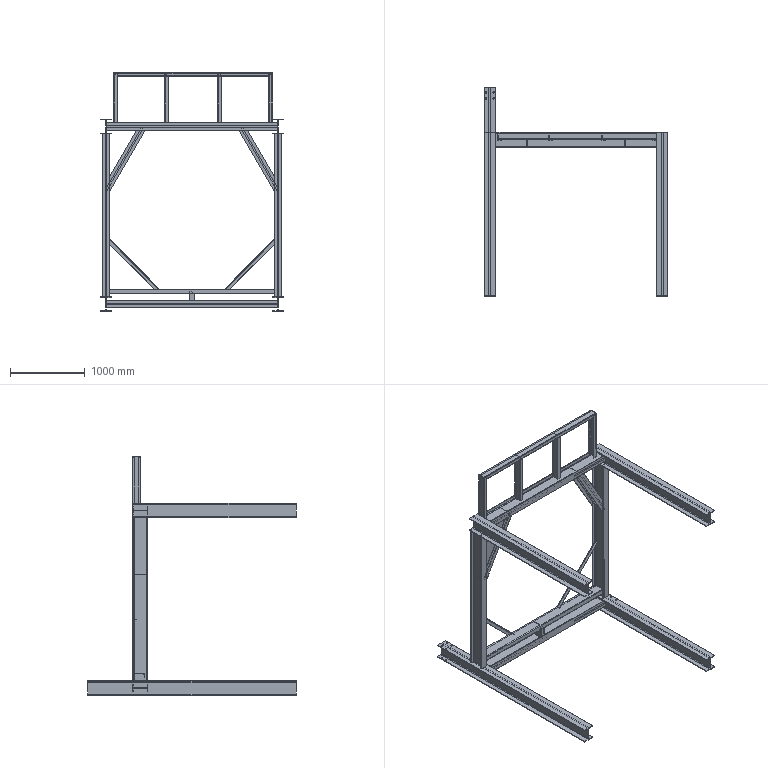Part | STEP file | 中转釜Bracket 6主体_Default<As Machined> | 19 solids | 405 faces | box 2450 x 2778 x 3187 mm | volume 76248404 mm3 | plane 307 | cylinder 98 | commonest cylinder face diameters 16 x40 19 x24 8.4 x10 17 x10 2.66 x4 10 x4